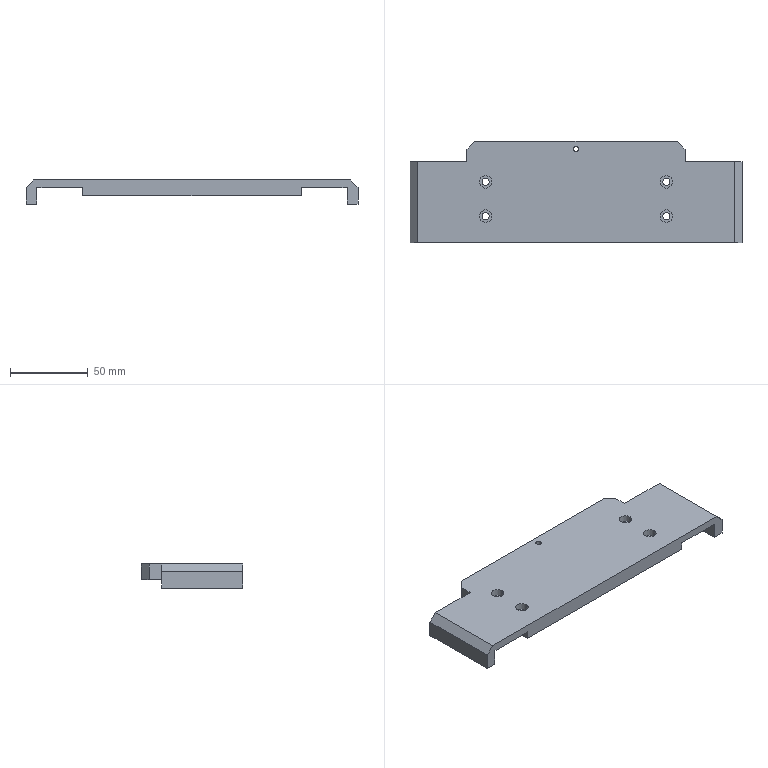Part | STEP file | (PA01.001.LX021) Stop Block B | 1 solid | 42 faces | box 213 x 65 x 15.5 mm | volume 114748 mm3 | plane 24 | cylinder 18 | commonest cylinder face diameters 4.5 x8 8 x8 3.3 x2